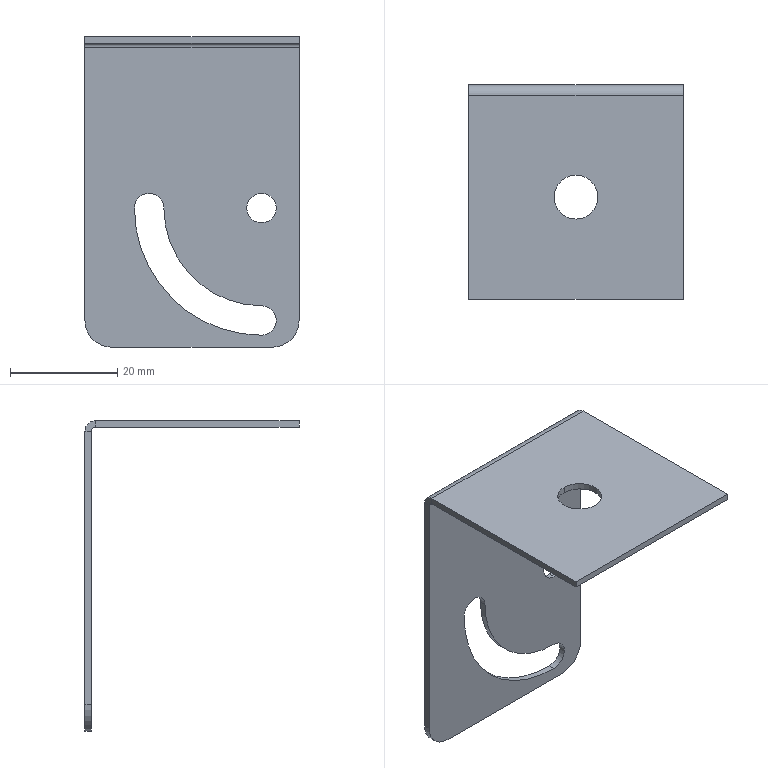Part | 1 solid | 25 faces | box 40 x 40 x 58 mm | volume 4268 mm3 | cylinder 13 | plane 12 | commonest cylinder face diameters 5.5 x5 8.2 x2 10 x2 1.473 x1 3.873 x1 36.5 x1
STEP:
#1=CARTESIAN_POINT('',(0.,-25.068,29.));
#2=VERTEX_POINT('',#1);
#3=CARTESIAN_POINT('',(0.,-16.868,29.));
#4=VERTEX_POINT('',#3);
#5=CARTESIAN_POINT('',(0.,-20.968,29.));
#6=DIRECTION('',(0.,0.,-1.));
#7=DIRECTION('',(0.,1.,0.));
#8=AXIS2_PLACEMENT_3D('',#5,#6,#7);
#9=CIRCLE('',#8,4.1);
#10=EDGE_CURVE('',#2,#4,#9,.T.);
#11=ORIENTED_EDGE('',*,*,#10,.F.);
#12=CARTESIAN_POINT('',(0.,-25.068,27.8));
#13=VERTEX_POINT('',#12);
#14=CARTESIAN_POINT('',(0.,-25.068,27.8));
#15=DIRECTION('',(0.,0.,-1.));
#16=VECTOR('',#15,1000.);
#17=LINE('',#14,#16);
#18=EDGE_CURVE('',#2,#13,#17,.T.);
#19=ORIENTED_EDGE('',*,*,#18,.T.);
#20=CARTESIAN_POINT('',(0.,-16.868,27.8));
#21=VERTEX_POINT('',#20);
#22=CARTESIAN_POINT('',(0.,-20.968,27.8));
#23=DIRECTION('',(0.,0.,-1.));
#24=DIRECTION('',(0.,1.,0.));
#25=AXIS2_PLACEMENT_3D('',#22,#23,#24);
#26=CIRCLE('',#25,4.1);
#27=EDGE_CURVE('',#13,#21,#26,.T.);
#28=ORIENTED_EDGE('',*,*,#27,.T.);
#29=CARTESIAN_POINT('',(0.,-16.868,27.8));
#30=DIRECTION('',(0.,0.,-1.));
#31=VECTOR('',#30,1000.);
#32=LINE('',#29,#31);
#33=EDGE_CURVE('',#4,#21,#32,.T.);
#34=ORIENTED_EDGE('',*,*,#33,.F.);
#35=EDGE_LOOP('',(#11,#19,#28,#34));
#36=FACE_OUTER_BOUND('',#35,.T.);
#37=CARTESIAN_POINT('',(0.,-20.968,27.8));
#38=DIRECTION('',(0.,0.,-1.));
#39=DIRECTION('',(0.,1.,0.));
#40=AXIS2_PLACEMENT_3D('',#37,#38,#39);
#41=CYLINDRICAL_SURFACE('',#40,4.1);
#42=ADVANCED_FACE('',(#36),#41,.F.);
#43=CARTESIAN_POINT('',(-5.25,-1.2,-3.));
#44=VERTEX_POINT('',#43);
#45=CARTESIAN_POINT('',(-8.,-1.2,-0.25));
#46=VERTEX_POINT('',#45);
#47=CARTESIAN_POINT('',(-8.,-1.2,-3.));
#48=DIRECTION('',(0.,-1.,0.));
#49=DIRECTION('',(0.,0.,-1.));
#50=AXIS2_PLACEMENT_3D('',#47,#48,#49);
#51=CIRCLE('',#50,2.75);
#52=EDGE_CURVE('',#44,#46,#51,.T.);
#53=ORIENTED_EDGE('',*,*,#52,.T.);
#54=CARTESIAN_POINT('',(-8.,0.,-0.25));
#55=VERTEX_POINT('',#54);
#56=CARTESIAN_POINT('',(-8.,-40.,-0.25));
#57=DIRECTION('',(0.,1.,0.));
#58=VECTOR('',#57,1000.);
#59=LINE('',#56,#58);
#60=EDGE_CURVE('',#46,#55,#59,.T.);
#61=ORIENTED_EDGE('',*,*,#60,.T.);
#62=CARTESIAN_POINT('',(-5.25,0.,-3.));
#63=VERTEX_POINT('',#62);
#64=CARTESIAN_POINT('',(-8.,0.,-3.));
#65=DIRECTION('',(0.,1.,0.));
#66=DIRECTION('',(0.,0.,1.));
#67=AXIS2_PLACEMENT_3D('',#64,#65,#66);
#68=CIRCLE('',#67,2.75);
#69=EDGE_CURVE('',#55,#63,#68,.T.);
#70=ORIENTED_EDGE('',*,*,#69,.T.);
#71=CARTESIAN_POINT('',(-5.25,-40.,-3.));
#72=DIRECTION('',(0.,1.,0.));
#73=VECTOR('',#72,1000.);
#74=LINE('',#71,#73);
#75=EDGE_CURVE('',#44,#63,#74,.T.);
#76=ORIENTED_EDGE('',*,*,#75,.F.);
#77=EDGE_LOOP('',(#53,#61,#70,#76));
#78=FACE_OUTER_BOUND('',#77,.T.);
#79=CARTESIAN_POINT('',(-8.,-40.,-3.));
#80=DIRECTION('',(0.,1.,0.));
#81=DIRECTION('',(0.,0.,1.));
#82=AXIS2_PLACEMENT_3D('',#79,#80,#81);
#83=CYLINDRICAL_SURFACE('',#82,2.75);
#84=ADVANCED_FACE('',(#78),#83,.F.);
#85=CARTESIAN_POINT('',(13.,-1.2,-0.25));
#86=VERTEX_POINT('',#85);
#87=CARTESIAN_POINT('',(13.,-1.2,-5.75));
#88=VERTEX_POINT('',#87);
#89=CARTESIAN_POINT('',(13.,-1.2,-3.));
#90=DIRECTION('',(0.,-1.,0.));
#91=DIRECTION('',(0.,0.,-1.));
#92=AXIS2_PLACEMENT_3D('',#89,#90,#91);
#93=CIRCLE('',#92,2.75);
#94=EDGE_CURVE('',#86,#88,#93,.T.);
#95=ORIENTED_EDGE('',*,*,#94,.T.);
#96=CARTESIAN_POINT('',(13.,0.,-5.75));
#97=VERTEX_POINT('',#96);
#98=CARTESIAN_POINT('',(13.,0.,-5.75));
#99=DIRECTION('',(0.,1.,0.));
#100=VECTOR('',#99,1000.);
#101=LINE('',#98,#100);
#102=EDGE_CURVE('',#88,#97,#101,.T.);
#103=ORIENTED_EDGE('',*,*,#102,.T.);
#104=CARTESIAN_POINT('',(13.,0.,-0.25));
#105=VERTEX_POINT('',#104);
#106=CARTESIAN_POINT('',(13.,0.,-3.));
#107=DIRECTION('',(0.,1.,0.));
#108=DIRECTION('',(0.,0.,1.));
#109=AXIS2_PLACEMENT_3D('',#106,#107,#108);
#110=CIRCLE('',#109,2.75);
#111=EDGE_CURVE('',#97,#105,#110,.T.);
#112=ORIENTED_EDGE('',*,*,#111,.T.);
#113=CARTESIAN_POINT('',(13.,0.,-0.25));
#114=DIRECTION('',(0.,1.,0.));
#115=VECTOR('',#114,1000.);
#116=LINE('',#113,#115);
#117=EDGE_CURVE('',#86,#105,#116,.T.);
#118=ORIENTED_EDGE('',*,*,#117,.F.);
#119=EDGE_LOOP('',(#95,#103,#112,#118));
#120=FACE_OUTER_BOUND('',#119,.T.);
#121=CARTESIAN_POINT('',(13.,0.,-3.));
#122=DIRECTION('',(0.,1.,0.));
#123=DIRECTION('',(0.,0.,1.));
#124=AXIS2_PLACEMENT_3D('',#121,#122,#123);
#125=CYLINDRICAL_SURFACE('',#124,2.75);
#126=ADVANCED_FACE('',(#120),#125,.F.);
#127=CARTESIAN_POINT('',(20.,-1.937,29.));
#128=VERTEX_POINT('',#127);
#129=CARTESIAN_POINT('',(20.,-40.,29.));
#130=VERTEX_POINT('',#129);
#131=CARTESIAN_POINT('',(20.,-40.,29.));
#132=DIRECTION('',(0.,-1.,0.));
#133=VECTOR('',#132,1000.);
#134=LINE('',#131,#133);
#135=EDGE_CURVE('',#128,#130,#134,.T.);
#136=ORIENTED_EDGE('',*,*,#135,.F.);
#137=CARTESIAN_POINT('',(-20.,-1.937,29.));
#138=VERTEX_POINT('',#137);
#139=CARTESIAN_POINT('',(0.,-1.937,29.));
#140=DIRECTION('',(-1.,0.,0.));
#141=VECTOR('',#140,1000.);
#142=LINE('',#139,#141);
#143=EDGE_CURVE('',#128,#138,#142,.T.);
#144=ORIENTED_EDGE('',*,*,#143,.T.);
#145=CARTESIAN_POINT('',(-20.,-40.,29.));
#146=VERTEX_POINT('',#145);
#147=CARTESIAN_POINT('',(-20.,-1.2,29.));
#148=DIRECTION('',(0.,1.,0.));
#149=VECTOR('',#148,1000.);
#150=LINE('',#147,#149);
#151=EDGE_CURVE('',#146,#138,#150,.T.);
#152=ORIENTED_EDGE('',*,*,#151,.F.);
#153=CARTESIAN_POINT('',(-20.,-40.,29.));
#154=DIRECTION('',(-1.,0.,0.));
#155=VECTOR('',#154,1000.);
#156=LINE('',#153,#155);
#157=EDGE_CURVE('',#130,#146,#156,.T.);
#158=ORIENTED_EDGE('',*,*,#157,.F.);
#159=EDGE_LOOP('',(#136,#144,#152,#158));
#160=FACE_OUTER_BOUND('',#159,.T.);
#161=CARTESIAN_POINT('',(0.,-20.968,29.));
#162=DIRECTION('',(0.,0.,-1.));
#163=DIRECTION('',(0.,1.,0.));
#164=AXIS2_PLACEMENT_3D('',#161,#162,#163);
#165=CIRCLE('',#164,4.1);
#166=EDGE_CURVE('',#4,#2,#165,.T.);
#167=ORIENTED_EDGE('',*,*,#166,.T.);
#168=ORIENTED_EDGE('',*,*,#10,.T.);
#169=EDGE_LOOP('',(#167,#168));
#170=FACE_BOUND('',#169,.T.);
#171=CARTESIAN_POINT('',(0.,0.,29.));
#172=DIRECTION('',(0.,0.,1.));
#173=DIRECTION('',(0.,-1.,0.));
#174=AXIS2_PLACEMENT_3D('',#171,#172,#173);
#175=PLANE('',#174);
#176=ADVANCED_FACE('',(#160,#170),#175,.T.);
#177=CARTESIAN_POINT('',(20.,-1.937,27.8));
#178=VERTEX_POINT('',#177);
#179=CARTESIAN_POINT('',(-20.,-1.937,27.8));
#180=VERTEX_POINT('',#179);
#181=CARTESIAN_POINT('',(20.,-1.937,27.8));
#182=DIRECTION('',(-1.,0.,0.));
#183=VECTOR('',#182,1000.);
#184=LINE('',#181,#183);
#185=EDGE_CURVE('',#178,#180,#184,.T.);
#186=ORIENTED_EDGE('',*,*,#185,.F.);
#187=CARTESIAN_POINT('',(20.,-40.,27.8));
#188=VERTEX_POINT('',#187);
#189=CARTESIAN_POINT('',(20.,0.,27.8));
#190=DIRECTION('',(0.,-1.,0.));
#191=VECTOR('',#190,1000.);
#192=LINE('',#189,#191);
#193=EDGE_CURVE('',#178,#188,#192,.T.);
#194=ORIENTED_EDGE('',*,*,#193,.T.);
#195=CARTESIAN_POINT('',(-20.,-40.,27.8));
#196=VERTEX_POINT('',#195);
#197=CARTESIAN_POINT('',(0.,-40.,27.8));
#198=DIRECTION('',(-1.,0.,0.));
#199=VECTOR('',#198,1000.);
#200=LINE('',#197,#199);
#201=EDGE_CURVE('',#188,#196,#200,.T.);
#202=ORIENTED_EDGE('',*,*,#201,.T.);
#203=CARTESIAN_POINT('',(-20.,0.,27.8));
#204=DIRECTION('',(0.,1.,0.));
#205=VECTOR('',#204,1000.);
#206=LINE('',#203,#205);
#207=EDGE_CURVE('',#196,#180,#206,.T.);
#208=ORIENTED_EDGE('',*,*,#207,.T.);
#209=EDGE_LOOP('',(#186,#194,#202,#208));
#210=FACE_OUTER_BOUND('',#209,.T.);
#211=CARTESIAN_POINT('',(0.,-20.968,27.8));
#212=DIRECTION('',(0.,0.,-1.));
#213=DIRECTION('',(0.,1.,0.));
#214=AXIS2_PLACEMENT_3D('',#211,#212,#213);
#215=CIRCLE('',#214,4.1);
#216=EDGE_CURVE('',#21,#13,#215,.T.);
#217=ORIENTED_EDGE('',*,*,#216,.F.);
#218=ORIENTED_EDGE('',*,*,#27,.F.);
#219=EDGE_LOOP('',(#217,#218));
#220=FACE_BOUND('',#219,.T.);
#221=CARTESIAN_POINT('',(0.,0.,27.8));
#222=DIRECTION('',(0.,0.,1.));
#223=DIRECTION('',(0.,-1.,0.));
#224=AXIS2_PLACEMENT_3D('',#221,#222,#223);
#225=PLANE('',#224);
#226=ADVANCED_FACE('',(#210,#220),#225,.F.);
#227=CARTESIAN_POINT('',(-20.,0.,-24.));
#228=VERTEX_POINT('',#227);
#229=CARTESIAN_POINT('',(-20.,0.,27.063));
#230=VERTEX_POINT('',#229);
#231=CARTESIAN_POINT('',(-20.,0.,29.));
#232=DIRECTION('',(0.,0.,1.));
#233=VECTOR('',#232,1000.);
#234=LINE('',#231,#233);
#235=EDGE_CURVE('',#228,#230,#234,.T.);
#236=ORIENTED_EDGE('',*,*,#235,.F.);
#237=CARTESIAN_POINT('',(-20.,-1.2,-24.));
#238=VERTEX_POINT('',#237);
#239=CARTESIAN_POINT('',(-20.,-1.2,-24.));
#240=DIRECTION('',(0.,-1.,0.));
#241=VECTOR('',#240,1000.);
#242=LINE('',#239,#241);
#243=EDGE_CURVE('',#228,#238,#242,.T.);
#244=ORIENTED_EDGE('',*,*,#243,.T.);
#245=CARTESIAN_POINT('',(-20.,-1.2,27.063));
#246=VERTEX_POINT('',#245);
#247=CARTESIAN_POINT('',(-20.,-1.2,29.));
#248=DIRECTION('',(0.,0.,1.));
#249=VECTOR('',#248,1000.);
#250=LINE('',#247,#249);
#251=EDGE_CURVE('',#238,#246,#250,.T.);
#252=ORIENTED_EDGE('',*,*,#251,.T.);
#253=CARTESIAN_POINT('',(-20.,-1.2,27.063));
#254=DIRECTION('',(0.,1.,0.));
#255=VECTOR('',#254,1000.);
#256=LINE('',#253,#255);
#257=EDGE_CURVE('',#246,#230,#256,.T.);
#258=ORIENTED_EDGE('',*,*,#257,.T.);
#259=EDGE_LOOP('',(#236,#244,#252,#258));
#260=FACE_OUTER_BOUND('',#259,.T.);
#261=CARTESIAN_POINT('',(-20.,-1.2,29.));
#262=DIRECTION('',(-1.,0.,0.));
#263=DIRECTION('',(0.,0.,1.));
#264=AXIS2_PLACEMENT_3D('',#261,#262,#263);
#265=PLANE('',#264);
#266=ADVANCED_FACE('',(#260),#265,.T.);
#267=CARTESIAN_POINT('',(13.,-1.2,-21.25));
#268=VERTEX_POINT('',#267);
#269=CARTESIAN_POINT('',(13.,-1.2,-3.));
#270=DIRECTION('',(0.,1.,0.));
#271=DIRECTION('',(0.,0.,-1.));
#272=AXIS2_PLACEMENT_3D('',#269,#270,#271);
#273=CIRCLE('',#272,18.25);
#274=EDGE_CURVE('',#268,#44,#273,.T.);
#275=ORIENTED_EDGE('',*,*,#274,.F.);
#276=CARTESIAN_POINT('',(13.,-1.2,-26.75));
#277=VERTEX_POINT('',#276);
#278=CARTESIAN_POINT('',(13.,-1.2,-24.));
#279=DIRECTION('',(0.,-1.,0.));
#280=DIRECTION('',(0.,0.,-1.));
#281=AXIS2_PLACEMENT_3D('',#278,#279,#280);
#282=CIRCLE('',#281,2.75);
#283=EDGE_CURVE('',#277,#268,#282,.T.);
#284=ORIENTED_EDGE('',*,*,#283,.F.);
#285=CARTESIAN_POINT('',(-10.75,-1.2,-3.));
#286=VERTEX_POINT('',#285);
#287=CARTESIAN_POINT('',(13.,-1.2,-3.));
#288=DIRECTION('',(0.,-1.,0.));
#289=DIRECTION('',(0.,0.,-1.));
#290=AXIS2_PLACEMENT_3D('',#287,#288,#289);
#291=CIRCLE('',#290,23.75);
#292=EDGE_CURVE('',#286,#277,#291,.T.);
#293=ORIENTED_EDGE('',*,*,#292,.F.);
#294=CARTESIAN_POINT('',(-8.,-1.2,-3.));
#295=DIRECTION('',(0.,-1.,0.));
#296=DIRECTION('',(0.,0.,-1.));
#297=AXIS2_PLACEMENT_3D('',#294,#295,#296);
#298=CIRCLE('',#297,2.75);
#299=EDGE_CURVE('',#46,#286,#298,.T.);
#300=ORIENTED_EDGE('',*,*,#299,.F.);
#301=ORIENTED_EDGE('',*,*,#52,.F.);
#302=EDGE_LOOP('',(#275,#284,#293,#300,#301));
#303=FACE_BOUND('',#302,.T.);
#304=ORIENTED_EDGE('',*,*,#94,.F.);
#305=CARTESIAN_POINT('',(13.,-1.2,-3.));
#306=DIRECTION('',(0.,-1.,0.));
#307=DIRECTION('',(0.,0.,-1.));
#308=AXIS2_PLACEMENT_3D('',#305,#306,#307);
#309=CIRCLE('',#308,2.75);
#310=EDGE_CURVE('',#88,#86,#309,.T.);
#311=ORIENTED_EDGE('',*,*,#310,.F.);
#312=EDGE_LOOP('',(#304,#311));
#313=FACE_BOUND('',#312,.T.);
#314=ORIENTED_EDGE('',*,*,#251,.F.);
#315=CARTESIAN_POINT('',(-15.,-1.2,-29.));
#316=VERTEX_POINT('',#315);
#317=CARTESIAN_POINT('',(-15.,-1.2,-24.));
#318=DIRECTION('',(0.,-1.,0.));
#319=DIRECTION('',(0.,0.,-1.));
#320=AXIS2_PLACEMENT_3D('',#317,#318,#319);
#321=CIRCLE('',#320,5.);
#322=EDGE_CURVE('',#238,#316,#321,.T.);
#323=ORIENTED_EDGE('',*,*,#322,.T.);
#324=CARTESIAN_POINT('',(15.,-1.2,-29.));
#325=VERTEX_POINT('',#324);
#326=CARTESIAN_POINT('',(-20.,-1.2,-29.));
#327=DIRECTION('',(-1.,0.,0.));
#328=VECTOR('',#327,1000.);
#329=LINE('',#326,#328);
#330=EDGE_CURVE('',#325,#316,#329,.T.);
#331=ORIENTED_EDGE('',*,*,#330,.F.);
#332=CARTESIAN_POINT('',(20.,-1.2,-24.));
#333=VERTEX_POINT('',#332);
#334=CARTESIAN_POINT('',(15.,-1.2,-24.));
#335=DIRECTION('',(0.,-1.,0.));
#336=DIRECTION('',(0.,0.,-1.));
#337=AXIS2_PLACEMENT_3D('',#334,#335,#336);
#338=CIRCLE('',#337,5.);
#339=EDGE_CURVE('',#325,#333,#338,.T.);
#340=ORIENTED_EDGE('',*,*,#339,.T.);
#341=CARTESIAN_POINT('',(20.,-1.2,27.063));
#342=VERTEX_POINT('',#341);
#343=CARTESIAN_POINT('',(20.,-1.2,29.));
#344=DIRECTION('',(0.,0.,-1.));
#345=VECTOR('',#344,1000.);
#346=LINE('',#343,#345);
#347=EDGE_CURVE('',#342,#333,#346,.T.);
#348=ORIENTED_EDGE('',*,*,#347,.F.);
#349=CARTESIAN_POINT('',(-20.,-1.2,27.063));
#350=DIRECTION('',(1.,0.,0.));
#351=VECTOR('',#350,1000.);
#352=LINE('',#349,#351);
#353=EDGE_CURVE('',#246,#342,#352,.T.);
#354=ORIENTED_EDGE('',*,*,#353,.F.);
#355=EDGE_LOOP('',(#314,#323,#331,#340,#348,#354));
#356=FACE_OUTER_BOUND('',#355,.T.);
#357=CARTESIAN_POINT('',(0.,-1.2,0.));
#358=DIRECTION('',(0.,-1.,0.));
#359=DIRECTION('',(0.,0.,-1.));
#360=AXIS2_PLACEMENT_3D('',#357,#358,#359);
#361=PLANE('',#360);
#362=ADVANCED_FACE('',(#303,#313,#356),#361,.T.);
#363=CARTESIAN_POINT('',(13.,0.,-21.25));
#364=VERTEX_POINT('',#363);
#365=CARTESIAN_POINT('',(13.,0.,-26.75));
#366=VERTEX_POINT('',#365);
#367=CARTESIAN_POINT('',(13.,0.,-24.));
#368=DIRECTION('',(0.,1.,0.));
#369=DIRECTION('',(0.,0.,1.));
#370=AXIS2_PLACEMENT_3D('',#367,#368,#369);
#371=CIRCLE('',#370,2.75);
#372=EDGE_CURVE('',#364,#366,#371,.T.);
#373=ORIENTED_EDGE('',*,*,#372,.F.);
#374=CARTESIAN_POINT('',(13.,0.,-3.));
#375=DIRECTION('',(0.,-1.,0.));
#376=DIRECTION('',(0.,0.,1.));
#377=AXIS2_PLACEMENT_3D('',#374,#375,#376);
#378=CIRCLE('',#377,18.25);
#379=EDGE_CURVE('',#63,#364,#378,.T.);
#380=ORIENTED_EDGE('',*,*,#379,.F.);
#381=ORIENTED_EDGE('',*,*,#69,.F.);
#382=CARTESIAN_POINT('',(-10.75,0.,-3.));
#383=VERTEX_POINT('',#382);
#384=CARTESIAN_POINT('',(-8.,0.,-3.));
#385=DIRECTION('',(0.,1.,0.));
#386=DIRECTION('',(0.,0.,1.));
#387=AXIS2_PLACEMENT_3D('',#384,#385,#386);
#388=CIRCLE('',#387,2.75);
#389=EDGE_CURVE('',#383,#55,#388,.T.);
#390=ORIENTED_EDGE('',*,*,#389,.F.);
#391=CARTESIAN_POINT('',(13.,0.,-3.));
#392=DIRECTION('',(0.,1.,0.));
#393=DIRECTION('',(0.,0.,1.));
#394=AXIS2_PLACEMENT_3D('',#391,#392,#393);
#395=CIRCLE('',#394,23.75);
#396=EDGE_CURVE('',#366,#383,#395,.T.);
#397=ORIENTED_EDGE('',*,*,#396,.F.);
#398=EDGE_LOOP('',(#373,#380,#381,#390,#397));
#399=FACE_BOUND('',#398,.T.);
#400=CARTESIAN_POINT('',(13.,0.,-3.));
#401=DIRECTION('',(0.,1.,0.));
#402=DIRECTION('',(0.,0.,1.));
#403=AXIS2_PLACEMENT_3D('',#400,#401,#402);
#404=CIRCLE('',#403,2.75);
#405=EDGE_CURVE('',#105,#97,#404,.T.);
#406=ORIENTED_EDGE('',*,*,#405,.F.);
#407=ORIENTED_EDGE('',*,*,#111,.F.);
#408=EDGE_LOOP('',(#406,#407));
#409=FACE_BOUND('',#408,.T.);
#410=CARTESIAN_POINT('',(15.,0.,-29.));
#411=VERTEX_POINT('',#410);
#412=CARTESIAN_POINT('',(-15.,0.,-29.));
#413=VERTEX_POINT('',#412);
#414=CARTESIAN_POINT('',(-20.,0.,-29.));
#415=DIRECTION('',(-1.,0.,0.));
#416=VECTOR('',#415,1000.);
#417=LINE('',#414,#416);
#418=EDGE_CURVE('',#411,#413,#417,.T.);
#419=ORIENTED_EDGE('',*,*,#418,.T.);
#420=CARTESIAN_POINT('',(-15.,0.,-24.));
#421=DIRECTION('',(0.,1.,0.));
#422=DIRECTION('',(0.,0.,-1.));
#423=AXIS2_PLACEMENT_3D('',#420,#421,#422);
#424=CIRCLE('',#423,5.);
#425=EDGE_CURVE('',#413,#228,#424,.T.);
#426=ORIENTED_EDGE('',*,*,#425,.T.);
#427=ORIENTED_EDGE('',*,*,#235,.T.);
#428=CARTESIAN_POINT('',(20.,0.,27.063));
#429=VERTEX_POINT('',#428);
#430=CARTESIAN_POINT('',(-20.,0.,27.063));
#431=DIRECTION('',(1.,0.,0.));
#432=VECTOR('',#431,1000.);
#433=LINE('',#430,#432);
#434=EDGE_CURVE('',#230,#429,#433,.T.);
#435=ORIENTED_EDGE('',*,*,#434,.T.);
#436=CARTESIAN_POINT('',(20.,0.,-24.));
#437=VERTEX_POINT('',#436);
#438=CARTESIAN_POINT('',(20.,0.,29.));
#439=DIRECTION('',(0.,0.,-1.));
#440=VECTOR('',#439,1000.);
#441=LINE('',#438,#440);
#442=EDGE_CURVE('',#429,#437,#441,.T.);
#443=ORIENTED_EDGE('',*,*,#442,.T.);
#444=CARTESIAN_POINT('',(15.,0.,-24.));
#445=DIRECTION('',(0.,1.,0.));
#446=DIRECTION('',(0.,0.,-1.));
#447=AXIS2_PLACEMENT_3D('',#444,#445,#446);
#448=CIRCLE('',#447,5.);
#449=EDGE_CURVE('',#437,#411,#448,.T.);
#450=ORIENTED_EDGE('',*,*,#449,.T.);
#451=EDGE_LOOP('',(#419,#426,#427,#435,#443,#450));
#452=FACE_OUTER_BOUND('',#451,.T.);
#453=CARTESIAN_POINT('',(0.,0.,0.));
#454=DIRECTION('',(0.,-1.,0.));
#455=DIRECTION('',(0.,0.,-1.));
#456=AXIS2_PLACEMENT_3D('',#453,#454,#455);
#457=PLANE('',#456);
#458=ADVANCED_FACE('',(#399,#409,#452),#457,.F.);
#459=ORIENTED_EDGE('',*,*,#347,.T.);
#460=CARTESIAN_POINT('',(20.,-1.2,-24.));
#461=DIRECTION('',(0.,1.,0.));
#462=VECTOR('',#461,1000.);
#463=LINE('',#460,#462);
#464=EDGE_CURVE('',#333,#437,#463,.T.);
#465=ORIENTED_EDGE('',*,*,#464,.T.);
#466=ORIENTED_EDGE('',*,*,#442,.F.);
#467=CARTESIAN_POINT('',(20.,-1.2,27.063));
#468=DIRECTION('',(0.,1.,0.));
#469=VECTOR('',#468,1000.);
#470=LINE('',#467,#469);
#471=EDGE_CURVE('',#342,#429,#470,.T.);
#472=ORIENTED_EDGE('',*,*,#471,.F.);
#473=EDGE_LOOP('',(#459,#465,#466,#472));
#474=FACE_OUTER_BOUND('',#473,.T.);
#475=CARTESIAN_POINT('',(20.,-1.2,29.));
#476=DIRECTION('',(1.,0.,0.));
#477=DIRECTION('',(0.,0.,-1.));
#478=AXIS2_PLACEMENT_3D('',#475,#476,#477);
#479=PLANE('',#478);
#480=ADVANCED_FACE('',(#474),#479,.T.);
#481=ORIENTED_EDGE('',*,*,#330,.T.);
#482=CARTESIAN_POINT('',(-15.,-1.2,-29.));
#483=DIRECTION('',(0.,1.,0.));
#484=VECTOR('',#483,1000.);
#485=LINE('',#482,#484);
#486=EDGE_CURVE('',#316,#413,#485,.T.);
#487=ORIENTED_EDGE('',*,*,#486,.T.);
#488=ORIENTED_EDGE('',*,*,#418,.F.);
#489=CARTESIAN_POINT('',(15.,-1.2,-29.));
#490=DIRECTION('',(0.,-1.,0.));
#491=VECTOR('',#490,1000.);
#492=LINE('',#489,#491);
#493=EDGE_CURVE('',#411,#325,#492,.T.);
#494=ORIENTED_EDGE('',*,*,#493,.T.);
#495=EDGE_LOOP('',(#481,#487,#488,#494));
#496=FACE_OUTER_BOUND('',#495,.T.);
#497=CARTESIAN_POINT('',(-20.,-1.2,-29.));
#498=DIRECTION('',(0.,0.,-1.));
#499=DIRECTION('',(-1.,0.,0.));
#500=AXIS2_PLACEMENT_3D('',#497,#498,#499);
#501=PLANE('',#500);
#502=ADVANCED_FACE('',(#496),#501,.T.);
#503=CARTESIAN_POINT('',(20.,-1.937,29.));
#504=DIRECTION('',(0.,0.,1.));
#505=VECTOR('',#504,1000.);
#506=LINE('',#503,#505);
#507=EDGE_CURVE('',#178,#128,#506,.T.);
#508=ORIENTED_EDGE('',*,*,#507,.F.);
#509=CARTESIAN_POINT('',(20.,-1.937,27.063));
#510=DIRECTION('',(1.,0.,0.));
#511=DIRECTION('',(0.,0.,1.));
#512=AXIS2_PLACEMENT_3D('',#509,#510,#511);
#513=CIRCLE('',#512,0.7366);
#514=EDGE_CURVE('',#342,#178,#513,.T.);
#515=ORIENTED_EDGE('',*,*,#514,.F.);
#516=ORIENTED_EDGE('',*,*,#471,.T.);
#517=CARTESIAN_POINT('',(20.,-1.937,27.063));
#518=DIRECTION('',(1.,0.,0.));
#519=DIRECTION('',(0.,0.,1.));
#520=AXIS2_PLACEMENT_3D('',#517,#518,#519);
#521=CIRCLE('',#520,1.937);
#522=EDGE_CURVE('',#429,#128,#521,.T.);
#523=ORIENTED_EDGE('',*,*,#522,.T.);
#524=EDGE_LOOP('',(#508,#515,#516,#523));
#525=FACE_OUTER_BOUND('',#524,.T.);
#526=CARTESIAN_POINT('',(20.,-1.937,27.063));
#527=DIRECTION('',(1.,0.,0.));
#528=DIRECTION('',(0.,0.,-1.));
#529=AXIS2_PLACEMENT_3D('',#526,#527,#528);
#530=PLANE('',#529);
#531=ADVANCED_FACE('',(#525),#530,.T.);
#532=CARTESIAN_POINT('',(-20.,-1.937,27.063));
#533=DIRECTION('',(-1.,0.,0.));
#534=DIRECTION('',(0.,0.,1.));
#535=AXIS2_PLACEMENT_3D('',#532,#533,#534);
#536=CIRCLE('',#535,0.7366);
#537=EDGE_CURVE('',#180,#246,#536,.T.);
#538=ORIENTED_EDGE('',*,*,#537,.F.);
#539=CARTESIAN_POINT('',(-20.,-1.937,27.8));
#540=DIRECTION('',(0.,0.,1.));
#541=VECTOR('',#540,1000.);
#542=LINE('',#539,#541);
#543=EDGE_CURVE('',#180,#138,#542,.T.);
#544=ORIENTED_EDGE('',*,*,#543,.T.);
#545=CARTESIAN_POINT('',(-20.,-1.937,27.063));
#546=DIRECTION('',(-1.,0.,0.));
#547=DIRECTION('',(0.,0.,1.));
#548=AXIS2_PLACEMENT_3D('',#545,#546,#547);
#549=CIRCLE('',#548,1.937);
#550=EDGE_CURVE('',#138,#230,#549,.T.);
#551=ORIENTED_EDGE('',*,*,#550,.T.);
#552=ORIENTED_EDGE('',*,*,#257,.F.);
#553=EDGE_LOOP('',(#538,#544,#551,#552));
#554=FACE_OUTER_BOUND('',#553,.T.);
#555=CARTESIAN_POINT('',(-20.,-1.937,27.063));
#556=DIRECTION('',(1.,0.,0.));
#557=DIRECTION('',(0.,0.,-1.));
#558=AXIS2_PLACEMENT_3D('',#555,#556,#557);
#559=PLANE('',#558);
#560=ADVANCED_FACE('',(#554),#559,.F.);
#561=ORIENTED_EDGE('',*,*,#434,.F.);
#562=ORIENTED_EDGE('',*,*,#550,.F.);
#563=ORIENTED_EDGE('',*,*,#143,.F.);
#564=ORIENTED_EDGE('',*,*,#522,.F.);
#565=EDGE_LOOP('',(#561,#562,#563,#564));
#566=FACE_OUTER_BOUND('',#565,.T.);
#567=CARTESIAN_POINT('',(-20.,-1.937,27.063));
#568=DIRECTION('',(-1.,0.,0.));
#569=DIRECTION('',(0.,0.,1.));
#570=AXIS2_PLACEMENT_3D('',#567,#568,#569);
#571=CYLINDRICAL_SURFACE('',#570,1.937);
#572=ADVANCED_FACE('',(#566),#571,.T.);
#573=ORIENTED_EDGE('',*,*,#353,.T.);
#574=ORIENTED_EDGE('',*,*,#514,.T.);
#575=ORIENTED_EDGE('',*,*,#185,.T.);
#576=ORIENTED_EDGE('',*,*,#537,.T.);
#577=EDGE_LOOP('',(#573,#574,#575,#576));
#578=FACE_OUTER_BOUND('',#577,.T.);
#579=CARTESIAN_POINT('',(-20.,-1.937,27.063));
#580=DIRECTION('',(-1.,0.,0.));
#581=DIRECTION('',(0.,0.,1.));
#582=AXIS2_PLACEMENT_3D('',#579,#580,#581);
#583=CYLINDRICAL_SURFACE('',#582,0.7366);
#584=ADVANCED_FACE('',(#578),#583,.F.);
#585=ORIENTED_EDGE('',*,*,#151,.T.);
#586=ORIENTED_EDGE('',*,*,#543,.F.);
#587=ORIENTED_EDGE('',*,*,#207,.F.);
#588=CARTESIAN_POINT('',(-20.,-40.,29.));
#589=DIRECTION('',(0.,0.,-1.));
#590=VECTOR('',#589,1000.);
#591=LINE('',#588,#590);
#592=EDGE_CURVE('',#146,#196,#591,.T.);
#593=ORIENTED_EDGE('',*,*,#592,.F.);
#594=EDGE_LOOP('',(#585,#586,#587,#593));
#595=FACE_OUTER_BOUND('',#594,.T.);
#596=CARTESIAN_POINT('',(-20.,-1.2,29.));
#597=DIRECTION('',(-1.,0.,0.));
#598=DIRECTION('',(0.,-1.,0.));
#599=AXIS2_PLACEMENT_3D('',#596,#597,#598);
#600=PLANE('',#599);
#601=ADVANCED_FACE('',(#595),#600,.T.);
#602=ORIENTED_EDGE('',*,*,#193,.F.);
#603=ORIENTED_EDGE('',*,*,#507,.T.);
#604=ORIENTED_EDGE('',*,*,#135,.T.);
#605=CARTESIAN_POINT('',(20.,-40.,29.));
#606=DIRECTION('',(0.,0.,-1.));
#607=VECTOR('',#606,1000.);
#608=LINE('',#605,#607);
#609=EDGE_CURVE('',#130,#188,#608,.T.);
#610=ORIENTED_EDGE('',*,*,#609,.T.);
#611=EDGE_LOOP('',(#602,#603,#604,#610));
#612=FACE_OUTER_BOUND('',#611,.T.);
#613=CARTESIAN_POINT('',(20.,-40.,29.));
#614=DIRECTION('',(1.,0.,0.));
#615=DIRECTION('',(0.,1.,0.));
#616=AXIS2_PLACEMENT_3D('',#613,#614,#615);
#617=PLANE('',#616);
#618=ADVANCED_FACE('',(#612),#617,.T.);
#619=ORIENTED_EDGE('',*,*,#201,.F.);
#620=ORIENTED_EDGE('',*,*,#609,.F.);
#621=ORIENTED_EDGE('',*,*,#157,.T.);
#622=ORIENTED_EDGE('',*,*,#592,.T.);
#623=EDGE_LOOP('',(#619,#620,#621,#622));
#624=FACE_OUTER_BOUND('',#623,.T.);
#625=CARTESIAN_POINT('',(-20.,-40.,29.));
#626=DIRECTION('',(0.,-1.,0.));
#627=DIRECTION('',(0.,0.,-1.));
#628=AXIS2_PLACEMENT_3D('',#625,#626,#627);
#629=PLANE('',#628);
#630=ADVANCED_FACE('',(#624),#629,.T.);
#631=ORIENTED_EDGE('',*,*,#322,.F.);
#632=ORIENTED_EDGE('',*,*,#243,.F.);
#633=ORIENTED_EDGE('',*,*,#425,.F.);
#634=ORIENTED_EDGE('',*,*,#486,.F.);
#635=EDGE_LOOP('',(#631,#632,#633,#634));
#636=FACE_OUTER_BOUND('',#635,.T.);
#637=CARTESIAN_POINT('',(-15.,-1.2,-24.));
#638=DIRECTION('',(0.,1.,0.));
#639=DIRECTION('',(0.,0.,1.));
#640=AXIS2_PLACEMENT_3D('',#637,#638,#639);
#641=CYLINDRICAL_SURFACE('',#640,5.);
#642=ADVANCED_FACE('',(#636),#641,.T.);
#643=ORIENTED_EDGE('',*,*,#339,.F.);
#644=ORIENTED_EDGE('',*,*,#493,.F.);
#645=ORIENTED_EDGE('',*,*,#449,.F.);
#646=ORIENTED_EDGE('',*,*,#464,.F.);
#647=EDGE_LOOP('',(#643,#644,#645,#646));
#648=FACE_OUTER_BOUND('',#647,.T.);
#649=CARTESIAN_POINT('',(15.,-1.2,-24.));
#650=DIRECTION('',(0.,1.,0.));
#651=DIRECTION('',(0.,0.,1.));
#652=AXIS2_PLACEMENT_3D('',#649,#650,#651);
#653=CYLINDRICAL_SURFACE('',#652,5.);
#654=ADVANCED_FACE('',(#648),#653,.T.);
#655=ORIENTED_EDGE('',*,*,#102,.F.);
#656=ORIENTED_EDGE('',*,*,#310,.T.);
#657=ORIENTED_EDGE('',*,*,#117,.T.);
#658=ORIENTED_EDGE('',*,*,#405,.T.);
#659=EDGE_LOOP('',(#655,#656,#657,#658));
#660=FACE_OUTER_BOUND('',#659,.T.);
#661=CARTESIAN_POINT('',(13.,0.,-3.));
#662=DIRECTION('',(0.,1.,0.));
#663=DIRECTION('',(0.,0.,1.));
#664=AXIS2_PLACEMENT_3D('',#661,#662,#663);
#665=CYLINDRICAL_SURFACE('',#664,2.75);
#666=ADVANCED_FACE('',(#660),#665,.F.);
#667=ORIENTED_EDGE('',*,*,#283,.T.);
#668=CARTESIAN_POINT('',(13.,-20.,-21.25));
#669=DIRECTION('',(0.,1.,0.));
#670=VECTOR('',#669,1000.);
#671=LINE('',#668,#670);
#672=EDGE_CURVE('',#268,#364,#671,.T.);
#673=ORIENTED_EDGE('',*,*,#672,.T.);
#674=ORIENTED_EDGE('',*,*,#372,.T.);
#675=CARTESIAN_POINT('',(13.,-20.,-26.75));
#676=DIRECTION('',(0.,1.,0.));
#677=VECTOR('',#676,1000.);
#678=LINE('',#675,#677);
#679=EDGE_CURVE('',#277,#366,#678,.T.);
#680=ORIENTED_EDGE('',*,*,#679,.F.);
#681=EDGE_LOOP('',(#667,#673,#674,#680));
#682=FACE_OUTER_BOUND('',#681,.T.);
#683=CARTESIAN_POINT('',(13.,0.,-24.));
#684=DIRECTION('',(0.,1.,0.));
#685=DIRECTION('',(0.,0.,1.));
#686=AXIS2_PLACEMENT_3D('',#683,#684,#685);
#687=CYLINDRICAL_SURFACE('',#686,2.75);
#688=ADVANCED_FACE('',(#682),#687,.F.);
#689=ORIENTED_EDGE('',*,*,#274,.T.);
#690=ORIENTED_EDGE('',*,*,#75,.T.);
#691=ORIENTED_EDGE('',*,*,#379,.T.);
#692=ORIENTED_EDGE('',*,*,#672,.F.);
#693=EDGE_LOOP('',(#689,#690,#691,#692));
#694=FACE_OUTER_BOUND('',#693,.T.);
#695=CARTESIAN_POINT('',(13.,-40.,-3.));
#696=DIRECTION('',(0.,1.,0.));
#697=DIRECTION('',(0.,0.,1.));
#698=AXIS2_PLACEMENT_3D('',#695,#696,#697);
#699=CYLINDRICAL_SURFACE('',#698,18.25);
#700=ADVANCED_FACE('',(#694),#699,.T.);
#701=ORIENTED_EDGE('',*,*,#60,.F.);
#702=ORIENTED_EDGE('',*,*,#299,.T.);
#703=CARTESIAN_POINT('',(-10.75,-40.,-3.));
#704=DIRECTION('',(0.,1.,0.));
#705=VECTOR('',#704,1000.);
#706=LINE('',#703,#705);
#707=EDGE_CURVE('',#286,#383,#706,.T.);
#708=ORIENTED_EDGE('',*,*,#707,.T.);
#709=ORIENTED_EDGE('',*,*,#389,.T.);
#710=EDGE_LOOP('',(#701,#702,#708,#709));
#711=FACE_OUTER_BOUND('',#710,.T.);
#712=CARTESIAN_POINT('',(-8.,-40.,-3.));
#713=DIRECTION('',(0.,1.,0.));
#714=DIRECTION('',(0.,0.,1.));
#715=AXIS2_PLACEMENT_3D('',#712,#713,#714);
#716=CYLINDRICAL_SURFACE('',#715,2.75);
#717=ADVANCED_FACE('',(#711),#716,.F.);
#718=ORIENTED_EDGE('',*,*,#292,.T.);
#719=ORIENTED_EDGE('',*,*,#679,.T.);
#720=ORIENTED_EDGE('',*,*,#396,.T.);
#721=ORIENTED_EDGE('',*,*,#707,.F.);
#722=EDGE_LOOP('',(#718,#719,#720,#721));
#723=FACE_OUTER_BOUND('',#722,.T.);
#724=CARTESIAN_POINT('',(13.,-40.,-3.));
#725=DIRECTION('',(0.,1.,0.));
#726=DIRECTION('',(0.,0.,1.));
#727=AXIS2_PLACEMENT_3D('',#724,#725,#726);
#728=CYLINDRICAL_SURFACE('',#727,23.75);
#729=ADVANCED_FACE('',(#723),#728,.F.);
#730=ORIENTED_EDGE('',*,*,#18,.F.);
#731=ORIENTED_EDGE('',*,*,#166,.F.);
#732=ORIENTED_EDGE('',*,*,#33,.T.);
#733=ORIENTED_EDGE('',*,*,#216,.T.);
#734=EDGE_LOOP('',(#730,#731,#732,#733));
#735=FACE_OUTER_BOUND('',#734,.T.);
#736=CARTESIAN_POINT('',(0.,-20.968,27.8));
#737=DIRECTION('',(0.,0.,-1.));
#738=DIRECTION('',(0.,1.,0.));
#739=AXIS2_PLACEMENT_3D('',#736,#737,#738);
#740=CYLINDRICAL_SURFACE('',#739,4.1);
#741=ADVANCED_FACE('',(#735),#740,.F.);
#742=CLOSED_SHELL('',(#42,#84,#126,#176,#226,#266,#362,#458,#480,#502,#531,#560,#572,#584,#601,#618,#630,#642,#654,#666,#688,#700,#717,#729,#741));
#743=MANIFOLD_SOLID_BREP('',#742);
#744=CARTESIAN_POINT('',(0.,0.,0.));
#745=DIRECTION('',(0.,0.,1.));
#746=DIRECTION('',(1.,0.,0.));
#747=AXIS2_PLACEMENT_3D('',#744,#745,#746);
#748=(LENGTH_UNIT()NAMED_UNIT(*)SI_UNIT(.MILLI.,.METRE.));
#749=UNCERTAINTY_MEASURE_WITH_UNIT(LENGTH_MEASURE(0.00001),#748,'','');
#750=(NAMED_UNIT(*)PLANE_ANGLE_UNIT()SI_UNIT($,.RADIAN.));
#751=(NAMED_UNIT(*)SI_UNIT($,.STERADIAN.)SOLID_ANGLE_UNIT());
#752=(GEOMETRIC_REPRESENTATION_CONTEXT(3)GLOBAL_UNCERTAINTY_ASSIGNED_CONTEXT((#749))GLOBAL_UNIT_ASSIGNED_CONTEXT((#748,#750,#751))REPRESENTATION_CONTEXT('',''));
#753=ADVANCED_BREP_SHAPE_REPRESENTATION('',(#743,#747),#752);